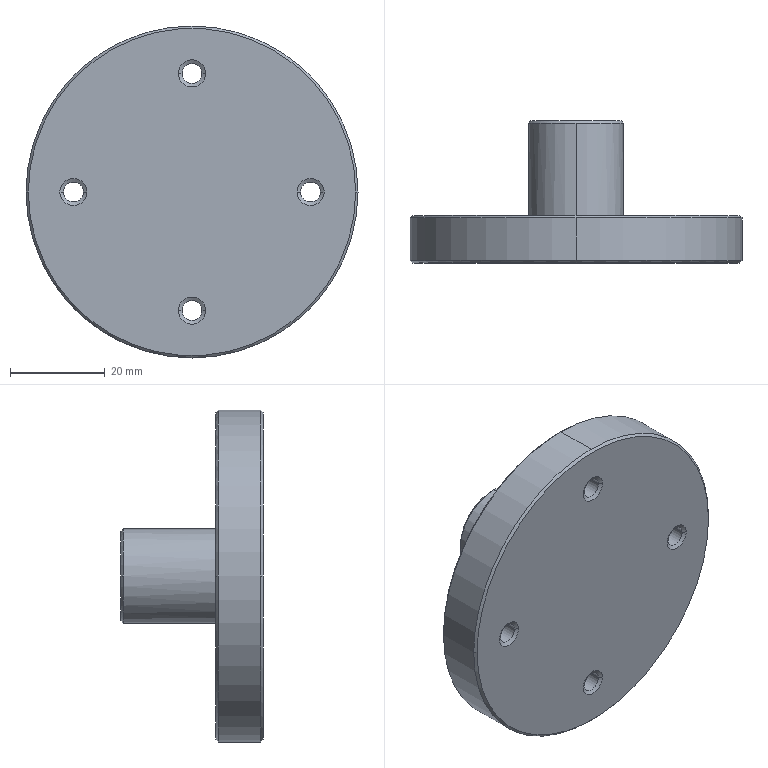Part | NX | 1 solid | 29 faces | box 70 x 30 x 70 mm | volume 44141 mm3 | cone 14 | cylinder 12 | plane 3 | commonest cylinder face diameters 4.2 x8 20 x2 70 x2
STEP:
#1=CARTESIAN_POINT('',(-9.5,30.,0.));
#2=VERTEX_POINT('',#1);
#3=CARTESIAN_POINT('',(9.5,30.,0.));
#4=VERTEX_POINT('',#3);
#5=CARTESIAN_POINT('',(0.,30.,0.));
#6=DIRECTION('',(0.,-1.,0.));
#7=DIRECTION('',(0.,0.,1.));
#8=AXIS2_PLACEMENT_3D('',#5,#6,#7);
#9=CIRCLE('',#8,9.5);
#10=EDGE_CURVE('',#2,#4,#9,.T.);
#11=ORIENTED_EDGE('',*,*,#10,.F.);
#12=CARTESIAN_POINT('',(0.,30.,0.));
#13=DIRECTION('',(0.,-1.,0.));
#14=DIRECTION('',(0.,0.,1.));
#15=AXIS2_PLACEMENT_3D('',#12,#13,#14);
#16=CIRCLE('',#15,9.5);
#17=EDGE_CURVE('',#4,#2,#16,.T.);
#18=ORIENTED_EDGE('',*,*,#17,.F.);
#19=EDGE_LOOP('',(#11,#18));
#20=FACE_BOUND('',#19,.T.);
#21=CARTESIAN_POINT('',(0.,30.,0.));
#22=DIRECTION('',(0.,1.,0.));
#23=DIRECTION('',(1.,0.,0.));
#24=AXIS2_PLACEMENT_3D('',#21,#22,#23);
#25=PLANE('',#24);
#26=ADVANCED_FACE('',(#20),#25,.T.);
#27=ORIENTED_EDGE('',*,*,#10,.T.);
#28=CARTESIAN_POINT('',(10.,29.5,0.));
#29=VERTEX_POINT('',#28);
#30=CARTESIAN_POINT('',(9.75,29.75,0.));
#31=DIRECTION('',(0.7071,-0.7071,0.));
#32=VECTOR('',#31,1000.);
#33=LINE('',#30,#32);
#34=EDGE_CURVE('',#4,#29,#33,.T.);
#35=ORIENTED_EDGE('',*,*,#34,.T.);
#36=CARTESIAN_POINT('',(0.,29.5,-10.));
#37=VERTEX_POINT('',#36);
#38=CARTESIAN_POINT('',(0.,29.5,0.));
#39=DIRECTION('',(0.,-1.,0.));
#40=DIRECTION('',(0.,0.,1.));
#41=AXIS2_PLACEMENT_3D('',#38,#39,#40);
#42=CIRCLE('',#41,10.);
#43=EDGE_CURVE('',#37,#29,#42,.T.);
#44=ORIENTED_EDGE('',*,*,#43,.F.);
#45=CARTESIAN_POINT('',(-10.,29.5,0.));
#46=VERTEX_POINT('',#45);
#47=CARTESIAN_POINT('',(0.,29.5,0.));
#48=DIRECTION('',(0.,-1.,0.));
#49=DIRECTION('',(0.,0.,1.));
#50=AXIS2_PLACEMENT_3D('',#47,#48,#49);
#51=CIRCLE('',#50,10.);
#52=EDGE_CURVE('',#46,#37,#51,.T.);
#53=ORIENTED_EDGE('',*,*,#52,.F.);
#54=CARTESIAN_POINT('',(-9.75,29.75,0.));
#55=DIRECTION('',(-0.7071,-0.7071,0.));
#56=VECTOR('',#55,1000.);
#57=LINE('',#54,#56);
#58=EDGE_CURVE('',#2,#46,#57,.T.);
#59=ORIENTED_EDGE('',*,*,#58,.F.);
#60=EDGE_LOOP('',(#27,#35,#44,#53,#59));
#61=FACE_BOUND('',#60,.T.);
#62=CARTESIAN_POINT('',(0.,29.75,0.));
#63=DIRECTION('',(0.,-1.,0.));
#64=DIRECTION('',(-1.,0.,0.));
#65=AXIS2_PLACEMENT_3D('',#62,#63,#64);
#66=CONICAL_SURFACE('',#65,9.75,0.7854);
#67=ADVANCED_FACE('',(#61),#66,.T.);
#68=CARTESIAN_POINT('',(0.,10.,10.));
#69=VERTEX_POINT('',#68);
#70=CARTESIAN_POINT('',(0.,10.,-10.));
#71=VERTEX_POINT('',#70);
#72=CARTESIAN_POINT('',(0.,10.,0.));
#73=DIRECTION('',(0.,1.,0.));
#74=DIRECTION('',(0.,0.,1.));
#75=AXIS2_PLACEMENT_3D('',#72,#73,#74);
#76=CIRCLE('',#75,10.);
#77=EDGE_CURVE('',#69,#71,#76,.T.);
#78=ORIENTED_EDGE('',*,*,#77,.T.);
#79=CARTESIAN_POINT('',(0.,-1.5,-10.));
#80=DIRECTION('',(0.,1.,0.));
#81=VECTOR('',#80,1000.);
#82=LINE('',#79,#81);
#83=EDGE_CURVE('',#71,#37,#82,.T.);
#84=ORIENTED_EDGE('',*,*,#83,.T.);
#85=ORIENTED_EDGE('',*,*,#43,.T.);
#86=CARTESIAN_POINT('',(0.,29.5,10.));
#87=VERTEX_POINT('',#86);
#88=CARTESIAN_POINT('',(0.,29.5,0.));
#89=DIRECTION('',(0.,-1.,0.));
#90=DIRECTION('',(0.,0.,1.));
#91=AXIS2_PLACEMENT_3D('',#88,#89,#90);
#92=CIRCLE('',#91,10.);
#93=EDGE_CURVE('',#29,#87,#92,.T.);
#94=ORIENTED_EDGE('',*,*,#93,.T.);
#95=CARTESIAN_POINT('',(0.,-1.5,10.));
#96=DIRECTION('',(0.,1.,0.));
#97=VECTOR('',#96,1000.);
#98=LINE('',#95,#97);
#99=EDGE_CURVE('',#69,#87,#98,.T.);
#100=ORIENTED_EDGE('',*,*,#99,.F.);
#101=EDGE_LOOP('',(#78,#84,#85,#94,#100));
#102=FACE_BOUND('',#101,.T.);
#103=CARTESIAN_POINT('',(0.,-1.5,0.));
#104=DIRECTION('',(0.,1.,0.));
#105=DIRECTION('',(0.,0.,1.));
#106=AXIS2_PLACEMENT_3D('',#103,#104,#105);
#107=CYLINDRICAL_SURFACE('',#106,10.);
#108=ADVANCED_FACE('',(#102),#107,.T.);
#109=CARTESIAN_POINT('',(0.,0.5,35.));
#110=VERTEX_POINT('',#109);
#111=CARTESIAN_POINT('',(35.,0.5,0.));
#112=VERTEX_POINT('',#111);
#113=CARTESIAN_POINT('',(0.,0.5,0.));
#114=DIRECTION('',(0.,1.,0.));
#115=DIRECTION('',(0.,0.,1.));
#116=AXIS2_PLACEMENT_3D('',#113,#114,#115);
#117=CIRCLE('',#116,35.);
#118=EDGE_CURVE('',#110,#112,#117,.T.);
#119=ORIENTED_EDGE('',*,*,#118,.F.);
#120=CARTESIAN_POINT('',(-35.,0.5,0.));
#121=VERTEX_POINT('',#120);
#122=CARTESIAN_POINT('',(0.,0.5,0.));
#123=DIRECTION('',(0.,1.,0.));
#124=DIRECTION('',(0.,0.,1.));
#125=AXIS2_PLACEMENT_3D('',#122,#123,#124);
#126=CIRCLE('',#125,35.);
#127=EDGE_CURVE('',#121,#110,#126,.T.);
#128=ORIENTED_EDGE('',*,*,#127,.F.);
#129=CARTESIAN_POINT('',(-34.5,0.,0.));
#130=VERTEX_POINT('',#129);
#131=CARTESIAN_POINT('',(-34.75,0.25,0.));
#132=DIRECTION('',(-0.7071,0.7071,0.));
#133=VECTOR('',#132,1000.);
#134=LINE('',#131,#133);
#135=EDGE_CURVE('',#121,#130,#134,.F.);
#136=ORIENTED_EDGE('',*,*,#135,.T.);
#137=CARTESIAN_POINT('',(34.5,0.,0.));
#138=VERTEX_POINT('',#137);
#139=CARTESIAN_POINT('',(0.,0.,0.));
#140=DIRECTION('',(0.,1.,0.));
#141=DIRECTION('',(1.,0.,0.));
#142=AXIS2_PLACEMENT_3D('',#139,#140,#141);
#143=CIRCLE('',#142,34.5);
#144=EDGE_CURVE('',#130,#138,#143,.T.);
#145=ORIENTED_EDGE('',*,*,#144,.T.);
#146=CARTESIAN_POINT('',(34.75,0.25,0.));
#147=DIRECTION('',(0.7071,0.7071,0.));
#148=VECTOR('',#147,1000.);
#149=LINE('',#146,#148);
#150=EDGE_CURVE('',#112,#138,#149,.F.);
#151=ORIENTED_EDGE('',*,*,#150,.F.);
#152=EDGE_LOOP('',(#119,#128,#136,#145,#151));
#153=FACE_BOUND('',#152,.T.);
#154=CARTESIAN_POINT('',(0.,0.25,0.));
#155=DIRECTION('',(0.,1.,0.));
#156=DIRECTION('',(1.,0.,0.));
#157=AXIS2_PLACEMENT_3D('',#154,#155,#156);
#158=CONICAL_SURFACE('',#157,34.75,0.7854);
#159=ADVANCED_FACE('',(#153),#158,.T.);
#160=CARTESIAN_POINT('',(0.,0.,0.));
#161=DIRECTION('',(0.,1.,0.));
#162=DIRECTION('',(1.,0.,0.));
#163=AXIS2_PLACEMENT_3D('',#160,#161,#162);
#164=CIRCLE('',#163,34.5);
#165=EDGE_CURVE('',#138,#130,#164,.T.);
#166=ORIENTED_EDGE('',*,*,#165,.F.);
#167=ORIENTED_EDGE('',*,*,#144,.F.);
#168=EDGE_LOOP('',(#166,#167));
#169=FACE_BOUND('',#168,.T.);
#170=CARTESIAN_POINT('',(2.86,0.,-25.));
#171=VERTEX_POINT('',#170);
#172=CARTESIAN_POINT('',(-2.86,0.,-25.));
#173=VERTEX_POINT('',#172);
#174=CARTESIAN_POINT('',(0.,0.,-25.));
#175=DIRECTION('',(0.,-1.,0.));
#176=DIRECTION('',(-1.,0.,0.));
#177=AXIS2_PLACEMENT_3D('',#174,#175,#176);
#178=CIRCLE('',#177,2.86);
#179=EDGE_CURVE('',#171,#173,#178,.T.);
#180=ORIENTED_EDGE('',*,*,#179,.F.);
#181=CARTESIAN_POINT('',(0.,0.,-25.));
#182=DIRECTION('',(0.,-1.,0.));
#183=DIRECTION('',(-1.,0.,0.));
#184=AXIS2_PLACEMENT_3D('',#181,#182,#183);
#185=CIRCLE('',#184,2.86);
#186=EDGE_CURVE('',#173,#171,#185,.T.);
#187=ORIENTED_EDGE('',*,*,#186,.F.);
#188=EDGE_LOOP('',(#180,#187));
#189=FACE_BOUND('',#188,.T.);
#190=CARTESIAN_POINT('',(27.86,0.,0.));
#191=VERTEX_POINT('',#190);
#192=CARTESIAN_POINT('',(22.14,0.,0.));
#193=VERTEX_POINT('',#192);
#194=CARTESIAN_POINT('',(25.,0.,0.));
#195=DIRECTION('',(0.,-1.,0.));
#196=DIRECTION('',(-1.,0.,0.));
#197=AXIS2_PLACEMENT_3D('',#194,#195,#196);
#198=CIRCLE('',#197,2.86);
#199=EDGE_CURVE('',#191,#193,#198,.T.);
#200=ORIENTED_EDGE('',*,*,#199,.F.);
#201=CARTESIAN_POINT('',(25.,0.,0.));
#202=DIRECTION('',(0.,-1.,0.));
#203=DIRECTION('',(-1.,0.,0.));
#204=AXIS2_PLACEMENT_3D('',#201,#202,#203);
#205=CIRCLE('',#204,2.86);
#206=EDGE_CURVE('',#193,#191,#205,.T.);
#207=ORIENTED_EDGE('',*,*,#206,.F.);
#208=EDGE_LOOP('',(#200,#207));
#209=FACE_BOUND('',#208,.T.);
#210=CARTESIAN_POINT('',(-2.86,0.,25.));
#211=VERTEX_POINT('',#210);
#212=CARTESIAN_POINT('',(2.86,0.,25.));
#213=VERTEX_POINT('',#212);
#214=CARTESIAN_POINT('',(0.,0.,25.));
#215=DIRECTION('',(0.,-1.,0.));
#216=DIRECTION('',(-1.,0.,0.));
#217=AXIS2_PLACEMENT_3D('',#214,#215,#216);
#218=CIRCLE('',#217,2.86);
#219=EDGE_CURVE('',#211,#213,#218,.T.);
#220=ORIENTED_EDGE('',*,*,#219,.F.);
#221=CARTESIAN_POINT('',(0.,0.,25.));
#222=DIRECTION('',(0.,-1.,0.));
#223=DIRECTION('',(-1.,0.,0.));
#224=AXIS2_PLACEMENT_3D('',#221,#222,#223);
#225=CIRCLE('',#224,2.86);
#226=EDGE_CURVE('',#213,#211,#225,.T.);
#227=ORIENTED_EDGE('',*,*,#226,.F.);
#228=EDGE_LOOP('',(#220,#227));
#229=FACE_BOUND('',#228,.T.);
#230=CARTESIAN_POINT('',(-22.14,0.,0.));
#231=VERTEX_POINT('',#230);
#232=CARTESIAN_POINT('',(-27.86,0.,0.));
#233=VERTEX_POINT('',#232);
#234=CARTESIAN_POINT('',(-25.,0.,0.));
#235=DIRECTION('',(0.,-1.,0.));
#236=DIRECTION('',(-1.,0.,0.));
#237=AXIS2_PLACEMENT_3D('',#234,#235,#236);
#238=CIRCLE('',#237,2.86);
#239=EDGE_CURVE('',#231,#233,#238,.T.);
#240=ORIENTED_EDGE('',*,*,#239,.F.);
#241=CARTESIAN_POINT('',(-25.,0.,0.));
#242=DIRECTION('',(0.,-1.,0.));
#243=DIRECTION('',(-1.,0.,0.));
#244=AXIS2_PLACEMENT_3D('',#241,#242,#243);
#245=CIRCLE('',#244,2.86);
#246=EDGE_CURVE('',#233,#231,#245,.T.);
#247=ORIENTED_EDGE('',*,*,#246,.F.);
#248=EDGE_LOOP('',(#240,#247));
#249=FACE_BOUND('',#248,.T.);
#250=CARTESIAN_POINT('',(0.,0.,0.));
#251=DIRECTION('',(0.,1.,0.));
#252=DIRECTION('',(1.,0.,0.));
#253=AXIS2_PLACEMENT_3D('',#250,#251,#252);
#254=PLANE('',#253);
#255=ADVANCED_FACE('',(#169,#189,#209,#229,#249),#254,.F.);
#256=CARTESIAN_POINT('',(34.5,10.,0.));
#257=VERTEX_POINT('',#256);
#258=CARTESIAN_POINT('',(-34.5,10.,0.));
#259=VERTEX_POINT('',#258);
#260=CARTESIAN_POINT('',(0.,10.,0.));
#261=DIRECTION('',(0.,-1.,0.));
#262=DIRECTION('',(-1.,0.,0.));
#263=AXIS2_PLACEMENT_3D('',#260,#261,#262);
#264=CIRCLE('',#263,34.5);
#265=EDGE_CURVE('',#257,#259,#264,.T.);
#266=ORIENTED_EDGE('',*,*,#265,.F.);
#267=CARTESIAN_POINT('',(0.,10.,0.));
#268=DIRECTION('',(0.,-1.,0.));
#269=DIRECTION('',(-1.,0.,0.));
#270=AXIS2_PLACEMENT_3D('',#267,#268,#269);
#271=CIRCLE('',#270,34.5);
#272=EDGE_CURVE('',#259,#257,#271,.T.);
#273=ORIENTED_EDGE('',*,*,#272,.F.);
#274=EDGE_LOOP('',(#266,#273));
#275=FACE_BOUND('',#274,.T.);
#276=ORIENTED_EDGE('',*,*,#77,.F.);
#277=CARTESIAN_POINT('',(0.,10.,0.));
#278=DIRECTION('',(0.,1.,0.));
#279=DIRECTION('',(0.,0.,1.));
#280=AXIS2_PLACEMENT_3D('',#277,#278,#279);
#281=CIRCLE('',#280,10.);
#282=EDGE_CURVE('',#71,#69,#281,.T.);
#283=ORIENTED_EDGE('',*,*,#282,.F.);
#284=EDGE_LOOP('',(#276,#283));
#285=FACE_BOUND('',#284,.T.);
#286=CARTESIAN_POINT('',(2.1,10.,-25.));
#287=VERTEX_POINT('',#286);
#288=CARTESIAN_POINT('',(-2.1,10.,-25.));
#289=VERTEX_POINT('',#288);
#290=CARTESIAN_POINT('',(0.,10.,-25.));
#291=DIRECTION('',(0.,-1.,0.));
#292=DIRECTION('',(-1.,0.,0.));
#293=AXIS2_PLACEMENT_3D('',#290,#291,#292);
#294=CIRCLE('',#293,2.1);
#295=EDGE_CURVE('',#287,#289,#294,.T.);
#296=ORIENTED_EDGE('',*,*,#295,.T.);
#297=CARTESIAN_POINT('',(0.,10.,-25.));
#298=DIRECTION('',(0.,-1.,0.));
#299=DIRECTION('',(-1.,0.,0.));
#300=AXIS2_PLACEMENT_3D('',#297,#298,#299);
#301=CIRCLE('',#300,2.1);
#302=EDGE_CURVE('',#289,#287,#301,.T.);
#303=ORIENTED_EDGE('',*,*,#302,.T.);
#304=EDGE_LOOP('',(#296,#303));
#305=FACE_BOUND('',#304,.T.);
#306=CARTESIAN_POINT('',(-2.1,10.,25.));
#307=VERTEX_POINT('',#306);
#308=CARTESIAN_POINT('',(2.1,10.,25.));
#309=VERTEX_POINT('',#308);
#310=CARTESIAN_POINT('',(0.,10.,25.));
#311=DIRECTION('',(0.,-1.,0.));
#312=DIRECTION('',(-1.,0.,0.));
#313=AXIS2_PLACEMENT_3D('',#310,#311,#312);
#314=CIRCLE('',#313,2.1);
#315=EDGE_CURVE('',#307,#309,#314,.T.);
#316=ORIENTED_EDGE('',*,*,#315,.T.);
#317=CARTESIAN_POINT('',(0.,10.,25.));
#318=DIRECTION('',(0.,-1.,0.));
#319=DIRECTION('',(-1.,0.,0.));
#320=AXIS2_PLACEMENT_3D('',#317,#318,#319);
#321=CIRCLE('',#320,2.1);
#322=EDGE_CURVE('',#309,#307,#321,.T.);
#323=ORIENTED_EDGE('',*,*,#322,.T.);
#324=EDGE_LOOP('',(#316,#323));
#325=FACE_BOUND('',#324,.T.);
#326=CARTESIAN_POINT('',(-27.1,10.,0.));
#327=VERTEX_POINT('',#326);
#328=CARTESIAN_POINT('',(-22.9,10.,0.));
#329=VERTEX_POINT('',#328);
#330=CARTESIAN_POINT('',(-25.,10.,0.));
#331=DIRECTION('',(0.,-1.,0.));
#332=DIRECTION('',(-1.,0.,0.));
#333=AXIS2_PLACEMENT_3D('',#330,#331,#332);
#334=CIRCLE('',#333,2.1);
#335=EDGE_CURVE('',#327,#329,#334,.T.);
#336=ORIENTED_EDGE('',*,*,#335,.T.);
#337=CARTESIAN_POINT('',(-25.,10.,0.));
#338=DIRECTION('',(0.,-1.,0.));
#339=DIRECTION('',(-1.,0.,0.));
#340=AXIS2_PLACEMENT_3D('',#337,#338,#339);
#341=CIRCLE('',#340,2.1);
#342=EDGE_CURVE('',#329,#327,#341,.T.);
#343=ORIENTED_EDGE('',*,*,#342,.T.);
#344=EDGE_LOOP('',(#336,#343));
#345=FACE_BOUND('',#344,.T.);
#346=CARTESIAN_POINT('',(22.9,10.,0.));
#347=VERTEX_POINT('',#346);
#348=CARTESIAN_POINT('',(27.1,10.,0.));
#349=VERTEX_POINT('',#348);
#350=CARTESIAN_POINT('',(25.,10.,0.));
#351=DIRECTION('',(0.,-1.,0.));
#352=DIRECTION('',(-1.,0.,0.));
#353=AXIS2_PLACEMENT_3D('',#350,#351,#352);
#354=CIRCLE('',#353,2.1);
#355=EDGE_CURVE('',#347,#349,#354,.T.);
#356=ORIENTED_EDGE('',*,*,#355,.T.);
#357=CARTESIAN_POINT('',(25.,10.,0.));
#358=DIRECTION('',(0.,-1.,0.));
#359=DIRECTION('',(-1.,0.,0.));
#360=AXIS2_PLACEMENT_3D('',#357,#358,#359);
#361=CIRCLE('',#360,2.1);
#362=EDGE_CURVE('',#349,#347,#361,.T.);
#363=ORIENTED_EDGE('',*,*,#362,.T.);
#364=EDGE_LOOP('',(#356,#363));
#365=FACE_BOUND('',#364,.T.);
#366=CARTESIAN_POINT('',(0.,10.,0.));
#367=DIRECTION('',(0.,1.,0.));
#368=DIRECTION('',(1.,0.,0.));
#369=AXIS2_PLACEMENT_3D('',#366,#367,#368);
#370=PLANE('',#369);
#371=ADVANCED_FACE('',(#275,#285,#305,#325,#345,#365),#370,.T.);
#372=ORIENTED_EDGE('',*,*,#265,.T.);
#373=CARTESIAN_POINT('',(-35.,9.5,0.));
#374=VERTEX_POINT('',#373);
#375=CARTESIAN_POINT('',(-34.75,9.75,0.));
#376=DIRECTION('',(-0.7071,-0.7071,0.));
#377=VECTOR('',#376,1000.);
#378=LINE('',#375,#377);
#379=EDGE_CURVE('',#374,#259,#378,.F.);
#380=ORIENTED_EDGE('',*,*,#379,.F.);
#381=CARTESIAN_POINT('',(0.,9.5,35.));
#382=VERTEX_POINT('',#381);
#383=CARTESIAN_POINT('',(0.,9.5,0.));
#384=DIRECTION('',(0.,-1.,0.));
#385=DIRECTION('',(0.,0.,1.));
#386=AXIS2_PLACEMENT_3D('',#383,#384,#385);
#387=CIRCLE('',#386,35.);
#388=EDGE_CURVE('',#382,#374,#387,.T.);
#389=ORIENTED_EDGE('',*,*,#388,.F.);
#390=CARTESIAN_POINT('',(35.,9.5,0.));
#391=VERTEX_POINT('',#390);
#392=CARTESIAN_POINT('',(0.,9.5,0.));
#393=DIRECTION('',(0.,-1.,0.));
#394=DIRECTION('',(0.,0.,1.));
#395=AXIS2_PLACEMENT_3D('',#392,#393,#394);
#396=CIRCLE('',#395,35.);
#397=EDGE_CURVE('',#391,#382,#396,.T.);
#398=ORIENTED_EDGE('',*,*,#397,.F.);
#399=CARTESIAN_POINT('',(34.75,9.75,0.));
#400=DIRECTION('',(0.7071,-0.7071,0.));
#401=VECTOR('',#400,1000.);
#402=LINE('',#399,#401);
#403=EDGE_CURVE('',#391,#257,#402,.F.);
#404=ORIENTED_EDGE('',*,*,#403,.T.);
#405=EDGE_LOOP('',(#372,#380,#389,#398,#404));
#406=FACE_BOUND('',#405,.T.);
#407=CARTESIAN_POINT('',(0.,9.75,0.));
#408=DIRECTION('',(0.,-1.,0.));
#409=DIRECTION('',(-1.,0.,0.));
#410=AXIS2_PLACEMENT_3D('',#407,#408,#409);
#411=CONICAL_SURFACE('',#410,34.75,0.7854);
#412=ADVANCED_FACE('',(#406),#411,.T.);
#413=ORIENTED_EDGE('',*,*,#118,.T.);
#414=CARTESIAN_POINT('',(0.,0.5,-35.));
#415=VERTEX_POINT('',#414);
#416=CARTESIAN_POINT('',(0.,0.5,0.));
#417=DIRECTION('',(0.,1.,0.));
#418=DIRECTION('',(0.,0.,1.));
#419=AXIS2_PLACEMENT_3D('',#416,#417,#418);
#420=CIRCLE('',#419,35.);
#421=EDGE_CURVE('',#112,#415,#420,.T.);
#422=ORIENTED_EDGE('',*,*,#421,.T.);
#423=CARTESIAN_POINT('',(0.,9.5,-35.));
#424=VERTEX_POINT('',#423);
#425=CARTESIAN_POINT('',(0.,-1.5,-35.));
#426=DIRECTION('',(0.,1.,0.));
#427=VECTOR('',#426,1000.);
#428=LINE('',#425,#427);
#429=EDGE_CURVE('',#424,#415,#428,.F.);
#430=ORIENTED_EDGE('',*,*,#429,.F.);
#431=CARTESIAN_POINT('',(0.,9.5,0.));
#432=DIRECTION('',(0.,-1.,0.));
#433=DIRECTION('',(0.,0.,1.));
#434=AXIS2_PLACEMENT_3D('',#431,#432,#433);
#435=CIRCLE('',#434,35.);
#436=EDGE_CURVE('',#424,#391,#435,.T.);
#437=ORIENTED_EDGE('',*,*,#436,.T.);
#438=ORIENTED_EDGE('',*,*,#397,.T.);
#439=CARTESIAN_POINT('',(0.,-1.5,35.));
#440=DIRECTION('',(0.,1.,0.));
#441=VECTOR('',#440,1000.);
#442=LINE('',#439,#441);
#443=EDGE_CURVE('',#382,#110,#442,.F.);
#444=ORIENTED_EDGE('',*,*,#443,.T.);
#445=EDGE_LOOP('',(#413,#422,#430,#437,#438,#444));
#446=FACE_BOUND('',#445,.T.);
#447=CARTESIAN_POINT('',(0.,-1.5,0.));
#448=DIRECTION('',(0.,1.,0.));
#449=DIRECTION('',(0.,0.,1.));
#450=AXIS2_PLACEMENT_3D('',#447,#448,#449);
#451=CYLINDRICAL_SURFACE('',#450,35.);
#452=ADVANCED_FACE('',(#446),#451,.T.);
#453=ORIENTED_EDGE('',*,*,#295,.F.);
#454=CARTESIAN_POINT('',(2.1,0.4388,-25.));
#455=VERTEX_POINT('',#454);
#456=CARTESIAN_POINT('',(2.1,0.,-25.));
#457=DIRECTION('',(0.,-1.,0.));
#458=VECTOR('',#457,1000.);
#459=LINE('',#456,#458);
#460=EDGE_CURVE('',#287,#455,#459,.T.);
#461=ORIENTED_EDGE('',*,*,#460,.T.);
#462=CARTESIAN_POINT('',(-2.1,0.4388,-25.));
#463=VERTEX_POINT('',#462);
#464=CARTESIAN_POINT('',(0.,0.4388,-25.));
#465=DIRECTION('',(0.,-1.,0.));
#466=DIRECTION('',(-1.,0.,0.));
#467=AXIS2_PLACEMENT_3D('',#464,#465,#466);
#468=CIRCLE('',#467,2.1);
#469=EDGE_CURVE('',#455,#463,#468,.T.);
#470=ORIENTED_EDGE('',*,*,#469,.T.);
#471=CARTESIAN_POINT('',(-2.1,0.,-25.));
#472=DIRECTION('',(0.,-1.,0.));
#473=VECTOR('',#472,1000.);
#474=LINE('',#471,#473);
#475=EDGE_CURVE('',#289,#463,#474,.T.);
#476=ORIENTED_EDGE('',*,*,#475,.F.);
#477=EDGE_LOOP('',(#453,#461,#470,#476));
#478=FACE_BOUND('',#477,.T.);
#479=CARTESIAN_POINT('',(0.,0.,-25.));
#480=DIRECTION('',(0.,-1.,0.));
#481=DIRECTION('',(-1.,0.,0.));
#482=AXIS2_PLACEMENT_3D('',#479,#480,#481);
#483=CYLINDRICAL_SURFACE('',#482,2.1);
#484=ADVANCED_FACE('',(#478),#483,.F.);
#485=CARTESIAN_POINT('',(0.,0.4388,-25.));
#486=DIRECTION('',(0.,-1.,0.));
#487=DIRECTION('',(-1.,0.,0.));
#488=AXIS2_PLACEMENT_3D('',#485,#486,#487);
#489=CIRCLE('',#488,2.1);
#490=EDGE_CURVE('',#463,#455,#489,.T.);
#491=ORIENTED_EDGE('',*,*,#490,.F.);
#492=CARTESIAN_POINT('',(-2.1,0.4388,-25.));
#493=DIRECTION('',(-0.866,-0.5,0.));
#494=VECTOR('',#493,1000.);
#495=LINE('',#492,#494);
#496=EDGE_CURVE('',#173,#463,#495,.F.);
#497=ORIENTED_EDGE('',*,*,#496,.F.);
#498=ORIENTED_EDGE('',*,*,#186,.T.);
#499=CARTESIAN_POINT('',(2.1,0.4388,-25.));
#500=DIRECTION('',(0.866,-0.5,0.));
#501=VECTOR('',#500,1000.);
#502=LINE('',#499,#501);
#503=EDGE_CURVE('',#171,#455,#502,.F.);
#504=ORIENTED_EDGE('',*,*,#503,.T.);
#505=EDGE_LOOP('',(#491,#497,#498,#504));
#506=FACE_BOUND('',#505,.T.);
#507=CARTESIAN_POINT('',(0.,0.4388,-25.));
#508=DIRECTION('',(0.,-1.,0.));
#509=DIRECTION('',(-1.,0.,0.));
#510=AXIS2_PLACEMENT_3D('',#507,#508,#509);
#511=CONICAL_SURFACE('',#510,2.1,1.047);
#512=ADVANCED_FACE('',(#506),#511,.F.);
#513=ORIENTED_EDGE('',*,*,#315,.F.);
#514=CARTESIAN_POINT('',(-2.1,0.4388,25.));
#515=VERTEX_POINT('',#514);
#516=CARTESIAN_POINT('',(-2.1,0.,25.));
#517=DIRECTION('',(0.,-1.,0.));
#518=VECTOR('',#517,1000.);
#519=LINE('',#516,#518);
#520=EDGE_CURVE('',#515,#307,#519,.F.);
#521=ORIENTED_EDGE('',*,*,#520,.F.);
#522=CARTESIAN_POINT('',(2.1,0.4388,25.));
#523=VERTEX_POINT('',#522);
#524=CARTESIAN_POINT('',(0.,0.4388,25.));
#525=DIRECTION('',(0.,-1.,0.));
#526=DIRECTION('',(-1.,0.,0.));
#527=AXIS2_PLACEMENT_3D('',#524,#525,#526);
#528=CIRCLE('',#527,2.1);
#529=EDGE_CURVE('',#515,#523,#528,.T.);
#530=ORIENTED_EDGE('',*,*,#529,.T.);
#531=CARTESIAN_POINT('',(2.1,0.,25.));
#532=DIRECTION('',(0.,-1.,0.));
#533=VECTOR('',#532,1000.);
#534=LINE('',#531,#533);
#535=EDGE_CURVE('',#523,#309,#534,.F.);
#536=ORIENTED_EDGE('',*,*,#535,.T.);
#537=EDGE_LOOP('',(#513,#521,#530,#536));
#538=FACE_BOUND('',#537,.T.);
#539=CARTESIAN_POINT('',(0.,0.,25.));
#540=DIRECTION('',(0.,-1.,0.));
#541=DIRECTION('',(-1.,0.,0.));
#542=AXIS2_PLACEMENT_3D('',#539,#540,#541);
#543=CYLINDRICAL_SURFACE('',#542,2.1);
#544=ADVANCED_FACE('',(#538),#543,.F.);
#545=ORIENTED_EDGE('',*,*,#219,.T.);
#546=CARTESIAN_POINT('',(2.1,0.4388,25.));
#547=DIRECTION('',(0.866,-0.5,0.));
#548=VECTOR('',#547,1000.);
#549=LINE('',#546,#548);
#550=EDGE_CURVE('',#213,#523,#549,.F.);
#551=ORIENTED_EDGE('',*,*,#550,.T.);
#552=ORIENTED_EDGE('',*,*,#529,.F.);
#553=CARTESIAN_POINT('',(-2.1,0.4388,25.));
#554=DIRECTION('',(-0.866,-0.5,0.));
#555=VECTOR('',#554,1000.);
#556=LINE('',#553,#555);
#557=EDGE_CURVE('',#211,#515,#556,.F.);
#558=ORIENTED_EDGE('',*,*,#557,.F.);
#559=EDGE_LOOP('',(#545,#551,#552,#558));
#560=FACE_BOUND('',#559,.T.);
#561=CARTESIAN_POINT('',(0.,0.4388,25.));
#562=DIRECTION('',(0.,-1.,0.));
#563=DIRECTION('',(-1.,0.,0.));
#564=AXIS2_PLACEMENT_3D('',#561,#562,#563);
#565=CONICAL_SURFACE('',#564,2.1,1.047);
#566=ADVANCED_FACE('',(#560),#565,.F.);
#567=CARTESIAN_POINT('',(-27.1,0.4388,0.));
#568=VERTEX_POINT('',#567);
#569=CARTESIAN_POINT('',(-22.9,0.4388,0.));
#570=VERTEX_POINT('',#569);
#571=CARTESIAN_POINT('',(-25.,0.4388,0.));
#572=DIRECTION('',(0.,-1.,0.));
#573=DIRECTION('',(-1.,0.,0.));
#574=AXIS2_PLACEMENT_3D('',#571,#572,#573);
#575=CIRCLE('',#574,2.1);
#576=EDGE_CURVE('',#568,#570,#575,.T.);
#577=ORIENTED_EDGE('',*,*,#576,.T.);
#578=CARTESIAN_POINT('',(-22.9,0.,0.));
#579=DIRECTION('',(0.,-1.,0.));
#580=VECTOR('',#579,1000.);
#581=LINE('',#578,#580);
#582=EDGE_CURVE('',#570,#329,#581,.F.);
#583=ORIENTED_EDGE('',*,*,#582,.T.);
#584=ORIENTED_EDGE('',*,*,#335,.F.);
#585=CARTESIAN_POINT('',(-27.1,0.,0.));
#586=DIRECTION('',(0.,-1.,0.));
#587=VECTOR('',#586,1000.);
#588=LINE('',#585,#587);
#589=EDGE_CURVE('',#568,#327,#588,.F.);
#590=ORIENTED_EDGE('',*,*,#589,.F.);
#591=EDGE_LOOP('',(#577,#583,#584,#590));
#592=FACE_BOUND('',#591,.T.);
#593=CARTESIAN_POINT('',(-25.,0.,0.));
#594=DIRECTION('',(0.,-1.,0.));
#595=DIRECTION('',(-1.,0.,0.));
#596=AXIS2_PLACEMENT_3D('',#593,#594,#595);
#597=CYLINDRICAL_SURFACE('',#596,2.1);
#598=ADVANCED_FACE('',(#592),#597,.F.);
#599=ORIENTED_EDGE('',*,*,#576,.F.);
#600=CARTESIAN_POINT('',(-27.1,0.4388,0.));
#601=DIRECTION('',(-0.866,-0.5,0.));
#602=VECTOR('',#601,1000.);
#603=LINE('',#600,#602);
#604=EDGE_CURVE('',#233,#568,#603,.F.);
#605=ORIENTED_EDGE('',*,*,#604,.F.);
#606=ORIENTED_EDGE('',*,*,#246,.T.);
#607=CARTESIAN_POINT('',(-22.9,0.4388,0.));
#608=DIRECTION('',(0.866,-0.5,0.));
#609=VECTOR('',#608,1000.);
#610=LINE('',#607,#609);
#611=EDGE_CURVE('',#231,#570,#610,.F.);
#612=ORIENTED_EDGE('',*,*,#611,.T.);
#613=EDGE_LOOP('',(#599,#605,#606,#612));
#614=FACE_BOUND('',#613,.T.);
#615=CARTESIAN_POINT('',(-25.,0.4388,0.));
#616=DIRECTION('',(0.,-1.,0.));
#617=DIRECTION('',(-1.,0.,0.));
#618=AXIS2_PLACEMENT_3D('',#615,#616,#617);
#619=CONICAL_SURFACE('',#618,2.1,1.047);
#620=ADVANCED_FACE('',(#614),#619,.F.);
#621=ORIENTED_EDGE('',*,*,#355,.F.);
#622=CARTESIAN_POINT('',(22.9,0.4388,0.));
#623=VERTEX_POINT('',#622);
#624=CARTESIAN_POINT('',(22.9,0.,0.));
#625=DIRECTION('',(0.,-1.,0.));
#626=VECTOR('',#625,1000.);
#627=LINE('',#624,#626);
#628=EDGE_CURVE('',#623,#347,#627,.F.);
#629=ORIENTED_EDGE('',*,*,#628,.F.);
#630=CARTESIAN_POINT('',(27.1,0.4388,0.));
#631=VERTEX_POINT('',#630);
#632=CARTESIAN_POINT('',(25.,0.4388,0.));
#633=DIRECTION('',(0.,-1.,0.));
#634=DIRECTION('',(-1.,0.,0.));
#635=AXIS2_PLACEMENT_3D('',#632,#633,#634);
#636=CIRCLE('',#635,2.1);
#637=EDGE_CURVE('',#623,#631,#636,.T.);
#638=ORIENTED_EDGE('',*,*,#637,.T.);
#639=CARTESIAN_POINT('',(27.1,0.,0.));
#640=DIRECTION('',(0.,-1.,0.));
#641=VECTOR('',#640,1000.);
#642=LINE('',#639,#641);
#643=EDGE_CURVE('',#631,#349,#642,.F.);
#644=ORIENTED_EDGE('',*,*,#643,.T.);
#645=EDGE_LOOP('',(#621,#629,#638,#644));
#646=FACE_BOUND('',#645,.T.);
#647=CARTESIAN_POINT('',(25.,0.,0.));
#648=DIRECTION('',(0.,-1.,0.));
#649=DIRECTION('',(-1.,0.,0.));
#650=AXIS2_PLACEMENT_3D('',#647,#648,#649);
#651=CYLINDRICAL_SURFACE('',#650,2.1);
#652=ADVANCED_FACE('',(#646),#651,.F.);
#653=CARTESIAN_POINT('',(25.,0.4388,0.));
#654=DIRECTION('',(0.,-1.,0.));
#655=DIRECTION('',(-1.,0.,0.));
#656=AXIS2_PLACEMENT_3D('',#653,#654,#655);
#657=CIRCLE('',#656,2.1);
#658=EDGE_CURVE('',#631,#623,#657,.T.);
#659=ORIENTED_EDGE('',*,*,#658,.F.);
#660=CARTESIAN_POINT('',(27.1,0.4388,0.));
#661=DIRECTION('',(0.866,-0.5,0.));
#662=VECTOR('',#661,1000.);
#663=LINE('',#660,#662);
#664=EDGE_CURVE('',#191,#631,#663,.F.);
#665=ORIENTED_EDGE('',*,*,#664,.F.);
#666=ORIENTED_EDGE('',*,*,#199,.T.);
#667=CARTESIAN_POINT('',(22.9,0.4388,0.));
#668=DIRECTION('',(-0.866,-0.5,0.));
#669=VECTOR('',#668,1000.);
#670=LINE('',#667,#669);
#671=EDGE_CURVE('',#193,#623,#670,.F.);
#672=ORIENTED_EDGE('',*,*,#671,.T.);
#673=EDGE_LOOP('',(#659,#665,#666,#672));
#674=FACE_BOUND('',#673,.T.);
#675=CARTESIAN_POINT('',(25.,0.4388,0.));
#676=DIRECTION('',(0.,-1.,0.));
#677=DIRECTION('',(-1.,0.,0.));
#678=AXIS2_PLACEMENT_3D('',#675,#676,#677);
#679=CONICAL_SURFACE('',#678,2.1,1.047);
#680=ADVANCED_FACE('',(#674),#679,.F.);
#681=ORIENTED_EDGE('',*,*,#165,.T.);
#682=ORIENTED_EDGE('',*,*,#135,.F.);
#683=CARTESIAN_POINT('',(0.,0.5,0.));
#684=DIRECTION('',(0.,1.,0.));
#685=DIRECTION('',(0.,0.,1.));
#686=AXIS2_PLACEMENT_3D('',#683,#684,#685);
#687=CIRCLE('',#686,35.);
#688=EDGE_CURVE('',#415,#121,#687,.T.);
#689=ORIENTED_EDGE('',*,*,#688,.F.);
#690=ORIENTED_EDGE('',*,*,#421,.F.);
#691=ORIENTED_EDGE('',*,*,#150,.T.);
#692=EDGE_LOOP('',(#681,#682,#689,#690,#691));
#693=FACE_BOUND('',#692,.T.);
#694=CARTESIAN_POINT('',(0.,0.25,0.));
#695=DIRECTION('',(0.,1.,0.));
#696=DIRECTION('',(1.,0.,0.));
#697=AXIS2_PLACEMENT_3D('',#694,#695,#696);
#698=CONICAL_SURFACE('',#697,34.75,0.7854);
#699=ADVANCED_FACE('',(#693),#698,.T.);
#700=ORIENTED_EDGE('',*,*,#520,.T.);
#701=ORIENTED_EDGE('',*,*,#322,.F.);
#702=ORIENTED_EDGE('',*,*,#535,.F.);
#703=CARTESIAN_POINT('',(0.,0.4388,25.));
#704=DIRECTION('',(0.,-1.,0.));
#705=DIRECTION('',(-1.,0.,0.));
#706=AXIS2_PLACEMENT_3D('',#703,#704,#705);
#707=CIRCLE('',#706,2.1);
#708=EDGE_CURVE('',#523,#515,#707,.T.);
#709=ORIENTED_EDGE('',*,*,#708,.T.);
#710=EDGE_LOOP('',(#700,#701,#702,#709));
#711=FACE_BOUND('',#710,.T.);
#712=CARTESIAN_POINT('',(0.,0.,25.));
#713=DIRECTION('',(0.,-1.,0.));
#714=DIRECTION('',(-1.,0.,0.));
#715=AXIS2_PLACEMENT_3D('',#712,#713,#714);
#716=CYLINDRICAL_SURFACE('',#715,2.1);
#717=ADVANCED_FACE('',(#711),#716,.F.);
#718=ORIENTED_EDGE('',*,*,#671,.F.);
#719=ORIENTED_EDGE('',*,*,#206,.T.);
#720=ORIENTED_EDGE('',*,*,#664,.T.);
#721=ORIENTED_EDGE('',*,*,#637,.F.);
#722=EDGE_LOOP('',(#718,#719,#720,#721));
#723=FACE_BOUND('',#722,.T.);
#724=CARTESIAN_POINT('',(25.,0.4388,0.));
#725=DIRECTION('',(0.,-1.,0.));
#726=DIRECTION('',(-1.,0.,0.));
#727=AXIS2_PLACEMENT_3D('',#724,#725,#726);
#728=CONICAL_SURFACE('',#727,2.1,1.047);
#729=ADVANCED_FACE('',(#723),#728,.F.);
#730=ORIENTED_EDGE('',*,*,#436,.F.);
#731=CARTESIAN_POINT('',(0.,9.5,0.));
#732=DIRECTION('',(0.,-1.,0.));
#733=DIRECTION('',(0.,0.,1.));
#734=AXIS2_PLACEMENT_3D('',#731,#732,#733);
#735=CIRCLE('',#734,35.);
#736=EDGE_CURVE('',#374,#424,#735,.T.);
#737=ORIENTED_EDGE('',*,*,#736,.F.);
#738=ORIENTED_EDGE('',*,*,#379,.T.);
#739=ORIENTED_EDGE('',*,*,#272,.T.);
#740=ORIENTED_EDGE('',*,*,#403,.F.);
#741=EDGE_LOOP('',(#730,#737,#738,#739,#740));
#742=FACE_BOUND('',#741,.T.);
#743=CARTESIAN_POINT('',(0.,9.75,0.));
#744=DIRECTION('',(0.,-1.,0.));
#745=DIRECTION('',(-1.,0.,0.));
#746=AXIS2_PLACEMENT_3D('',#743,#744,#745);
#747=CONICAL_SURFACE('',#746,34.75,0.7854);
#748=ADVANCED_FACE('',(#742),#747,.T.);
#749=ORIENTED_EDGE('',*,*,#34,.F.);
#750=ORIENTED_EDGE('',*,*,#17,.T.);
#751=ORIENTED_EDGE('',*,*,#58,.T.);
#752=CARTESIAN_POINT('',(0.,29.5,0.));
#753=DIRECTION('',(0.,-1.,0.));
#754=DIRECTION('',(0.,0.,1.));
#755=AXIS2_PLACEMENT_3D('',#752,#753,#754);
#756=CIRCLE('',#755,10.);
#757=EDGE_CURVE('',#87,#46,#756,.T.);
#758=ORIENTED_EDGE('',*,*,#757,.F.);
#759=ORIENTED_EDGE('',*,*,#93,.F.);
#760=EDGE_LOOP('',(#749,#750,#751,#758,#759));
#761=FACE_BOUND('',#760,.T.);
#762=CARTESIAN_POINT('',(0.,29.75,0.));
#763=DIRECTION('',(0.,-1.,0.));
#764=DIRECTION('',(-1.,0.,0.));
#765=AXIS2_PLACEMENT_3D('',#762,#763,#764);
#766=CONICAL_SURFACE('',#765,9.75,0.7854);
#767=ADVANCED_FACE('',(#761),#766,.T.);
#768=ORIENTED_EDGE('',*,*,#239,.T.);
#769=ORIENTED_EDGE('',*,*,#604,.T.);
#770=CARTESIAN_POINT('',(-25.,0.4388,0.));
#771=DIRECTION('',(0.,-1.,0.));
#772=DIRECTION('',(-1.,0.,0.));
#773=AXIS2_PLACEMENT_3D('',#770,#771,#772);
#774=CIRCLE('',#773,2.1);
#775=EDGE_CURVE('',#570,#568,#774,.T.);
#776=ORIENTED_EDGE('',*,*,#775,.F.);
#777=ORIENTED_EDGE('',*,*,#611,.F.);
#778=EDGE_LOOP('',(#768,#769,#776,#777));
#779=FACE_BOUND('',#778,.T.);
#780=CARTESIAN_POINT('',(-25.,0.4388,0.));
#781=DIRECTION('',(0.,-1.,0.));
#782=DIRECTION('',(-1.,0.,0.));
#783=AXIS2_PLACEMENT_3D('',#780,#781,#782);
#784=CONICAL_SURFACE('',#783,2.1,1.047);
#785=ADVANCED_FACE('',(#779),#784,.F.);
#786=ORIENTED_EDGE('',*,*,#658,.T.);
#787=ORIENTED_EDGE('',*,*,#628,.T.);
#788=ORIENTED_EDGE('',*,*,#362,.F.);
#789=ORIENTED_EDGE('',*,*,#643,.F.);
#790=EDGE_LOOP('',(#786,#787,#788,#789));
#791=FACE_BOUND('',#790,.T.);
#792=CARTESIAN_POINT('',(25.,0.,0.));
#793=DIRECTION('',(0.,-1.,0.));
#794=DIRECTION('',(-1.,0.,0.));
#795=AXIS2_PLACEMENT_3D('',#792,#793,#794);
#796=CYLINDRICAL_SURFACE('',#795,2.1);
#797=ADVANCED_FACE('',(#791),#796,.F.);
#798=ORIENTED_EDGE('',*,*,#179,.T.);
#799=ORIENTED_EDGE('',*,*,#496,.T.);
#800=ORIENTED_EDGE('',*,*,#469,.F.);
#801=ORIENTED_EDGE('',*,*,#503,.F.);
#802=EDGE_LOOP('',(#798,#799,#800,#801));
#803=FACE_BOUND('',#802,.T.);
#804=CARTESIAN_POINT('',(0.,0.4388,-25.));
#805=DIRECTION('',(0.,-1.,0.));
#806=DIRECTION('',(-1.,0.,0.));
#807=AXIS2_PLACEMENT_3D('',#804,#805,#806);
#808=CONICAL_SURFACE('',#807,2.1,1.047);
#809=ADVANCED_FACE('',(#803),#808,.F.);
#810=ORIENTED_EDGE('',*,*,#429,.T.);
#811=ORIENTED_EDGE('',*,*,#688,.T.);
#812=ORIENTED_EDGE('',*,*,#127,.T.);
#813=ORIENTED_EDGE('',*,*,#443,.F.);
#814=ORIENTED_EDGE('',*,*,#388,.T.);
#815=ORIENTED_EDGE('',*,*,#736,.T.);
#816=EDGE_LOOP('',(#810,#811,#812,#813,#814,#815));
#817=FACE_BOUND('',#816,.T.);
#818=CARTESIAN_POINT('',(0.,-1.5,0.));
#819=DIRECTION('',(0.,1.,0.));
#820=DIRECTION('',(0.,0.,1.));
#821=AXIS2_PLACEMENT_3D('',#818,#819,#820);
#822=CYLINDRICAL_SURFACE('',#821,35.);
#823=ADVANCED_FACE('',(#817),#822,.T.);
#824=ORIENTED_EDGE('',*,*,#99,.T.);
#825=ORIENTED_EDGE('',*,*,#757,.T.);
#826=ORIENTED_EDGE('',*,*,#52,.T.);
#827=ORIENTED_EDGE('',*,*,#83,.F.);
#828=ORIENTED_EDGE('',*,*,#282,.T.);
#829=EDGE_LOOP('',(#824,#825,#826,#827,#828));
#830=FACE_BOUND('',#829,.T.);
#831=CARTESIAN_POINT('',(0.,-1.5,0.));
#832=DIRECTION('',(0.,1.,0.));
#833=DIRECTION('',(0.,0.,1.));
#834=AXIS2_PLACEMENT_3D('',#831,#832,#833);
#835=CYLINDRICAL_SURFACE('',#834,10.);
#836=ADVANCED_FACE('',(#830),#835,.T.);
#837=ORIENTED_EDGE('',*,*,#589,.T.);
#838=ORIENTED_EDGE('',*,*,#342,.F.);
#839=ORIENTED_EDGE('',*,*,#582,.F.);
#840=ORIENTED_EDGE('',*,*,#775,.T.);
#841=EDGE_LOOP('',(#837,#838,#839,#840));
#842=FACE_BOUND('',#841,.T.);
#843=CARTESIAN_POINT('',(-25.,0.,0.));
#844=DIRECTION('',(0.,-1.,0.));
#845=DIRECTION('',(-1.,0.,0.));
#846=AXIS2_PLACEMENT_3D('',#843,#844,#845);
#847=CYLINDRICAL_SURFACE('',#846,2.1);
#848=ADVANCED_FACE('',(#842),#847,.F.);
#849=ORIENTED_EDGE('',*,*,#557,.T.);
#850=ORIENTED_EDGE('',*,*,#708,.F.);
#851=ORIENTED_EDGE('',*,*,#550,.F.);
#852=ORIENTED_EDGE('',*,*,#226,.T.);
#853=EDGE_LOOP('',(#849,#850,#851,#852));
#854=FACE_BOUND('',#853,.T.);
#855=CARTESIAN_POINT('',(0.,0.4388,25.));
#856=DIRECTION('',(0.,-1.,0.));
#857=DIRECTION('',(-1.,0.,0.));
#858=AXIS2_PLACEMENT_3D('',#855,#856,#857);
#859=CONICAL_SURFACE('',#858,2.1,1.047);
#860=ADVANCED_FACE('',(#854),#859,.F.);
#861=ORIENTED_EDGE('',*,*,#490,.T.);
#862=ORIENTED_EDGE('',*,*,#460,.F.);
#863=ORIENTED_EDGE('',*,*,#302,.F.);
#864=ORIENTED_EDGE('',*,*,#475,.T.);
#865=EDGE_LOOP('',(#861,#862,#863,#864));
#866=FACE_BOUND('',#865,.T.);
#867=CARTESIAN_POINT('',(0.,0.,-25.));
#868=DIRECTION('',(0.,-1.,0.));
#869=DIRECTION('',(-1.,0.,0.));
#870=AXIS2_PLACEMENT_3D('',#867,#868,#869);
#871=CYLINDRICAL_SURFACE('',#870,2.1);
#872=ADVANCED_FACE('',(#866),#871,.F.);
#873=CLOSED_SHELL('',(#26,#67,#108,#159,#255,#371,#412,#452,#484,#512,#544,#566,#598,#620,#652,#680,#699,#717,#729,#748,#767,#785,#797,#809,#823,#836,#848,#860,#872));
#874=MANIFOLD_SOLID_BREP('',#873);
#875=(LENGTH_UNIT()NAMED_UNIT(*)SI_UNIT(.MILLI.,.METRE.));
#876=UNCERTAINTY_MEASURE_WITH_UNIT(LENGTH_MEASURE(0.00001),#875,'','');
#877=(NAMED_UNIT(*)PLANE_ANGLE_UNIT()SI_UNIT($,.RADIAN.));
#878=(NAMED_UNIT(*)SI_UNIT($,.STERADIAN.)SOLID_ANGLE_UNIT());
#879=(GEOMETRIC_REPRESENTATION_CONTEXT(3)GLOBAL_UNCERTAINTY_ASSIGNED_CONTEXT((#876))GLOBAL_UNIT_ASSIGNED_CONTEXT((#875,#877,#878))REPRESENTATION_CONTEXT('',''));
#880=ADVANCED_BREP_SHAPE_REPRESENTATION('',(#874),#879);